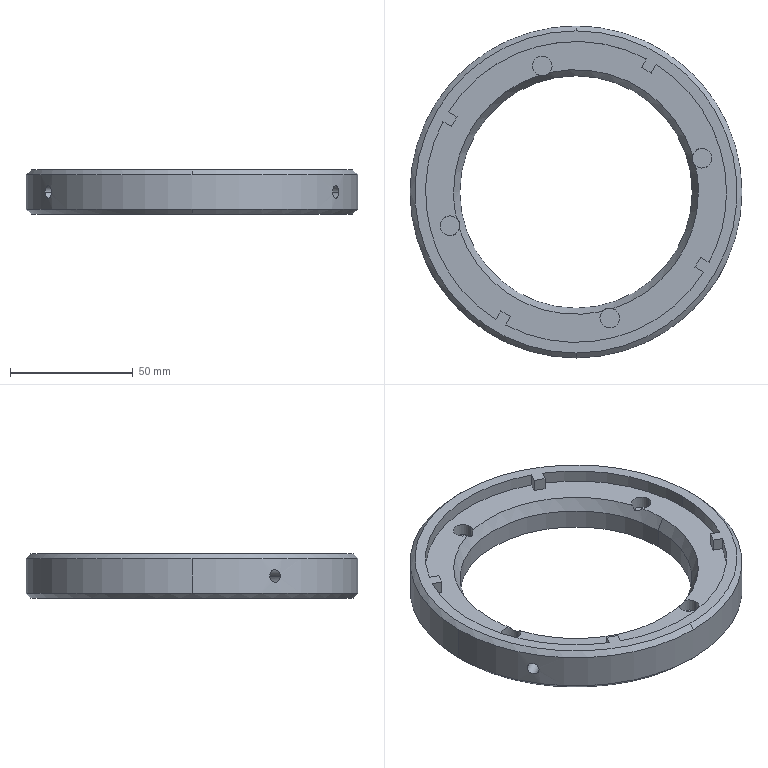Part | STEP file | Hub chuck-10P | 1 solid | 707 faces | box 135 x 135 x 18 mm | volume 101128 mm3 | plane 396 | spline 278 | cylinder 27 | cone 6 | commonest cylinder face diameters 8 x8 5 x6 122.4 x5 10 x4 94.5 x2 135 x2